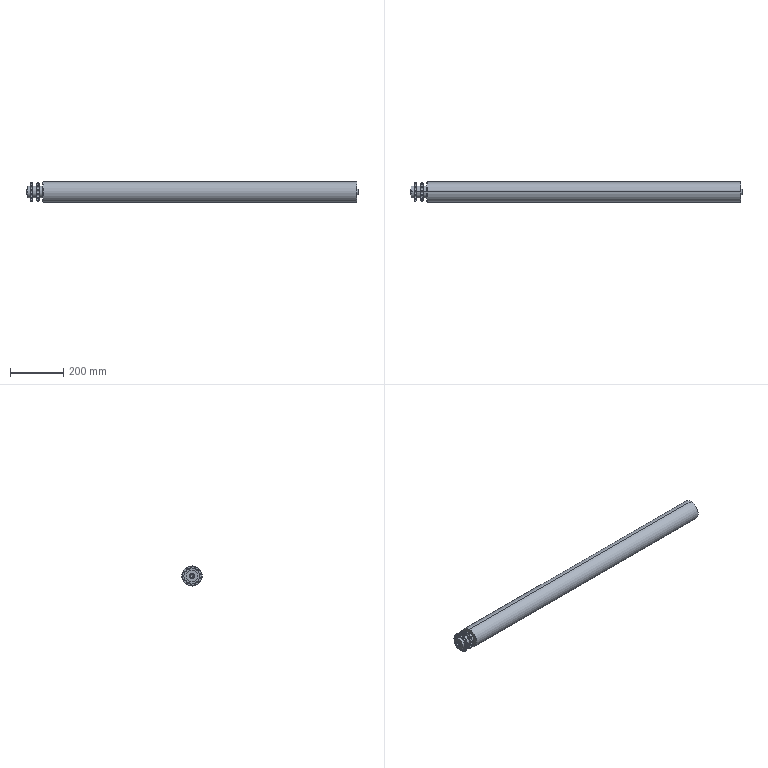Part | STEP file | 1 solid | 207 faces | box 1249 x 76 x 76 mm | volume 5468799 mm3 | cylinder 138 | spline 52 | plane 9 | cone 8 | commonest cylinder face diameters 16.701 x58 10.16 x38 73.939 x26 45 x6 10.2 x4 20 x4